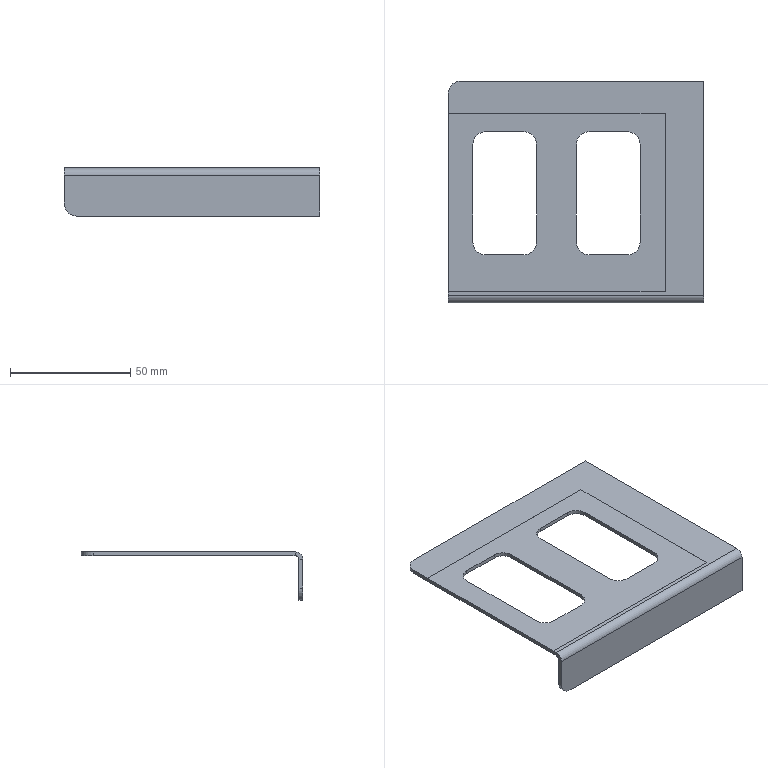Part | SolidWorks | features ICE 3, Fillet 1, FlatPattern 1, SMBaseFlange 1, SheetMetal 1 | 1 solid | 40 faces | box 106 x 92 x 20 mm | volume 14216 mm3 | plane 28 | cylinder 12 | commonest cylinder face diameters 10.4 x8 10 x2 3 x1 6.2 x1
STEP:
#1=CARTESIAN_POINT('',(15.4,19.9,-0.01));
#2=VERTEX_POINT('',#1);
#3=CARTESIAN_POINT('',(10.2,25.1,-0.01));
#4=VERTEX_POINT('',#3);
#5=CARTESIAN_POINT('',(15.4,25.1,-0.01));
#6=DIRECTION('',(0.,0.,-1.));
#7=DIRECTION('',(1.,0.,0.));
#8=AXIS2_PLACEMENT_3D('',#5,#6,#7);
#9=CIRCLE('',#8,5.2);
#10=EDGE_CURVE('',#2,#4,#9,.T.);
#11=ORIENTED_EDGE('',*,*,#10,.F.);
#12=CARTESIAN_POINT('',(15.4,19.9,-1.59));
#13=VERTEX_POINT('',#12);
#14=CARTESIAN_POINT('',(15.4,19.9,-20.001));
#15=DIRECTION('',(0.,0.,1.));
#16=VECTOR('',#15,1000.);
#17=LINE('',#14,#16);
#18=EDGE_CURVE('',#13,#2,#17,.T.);
#19=ORIENTED_EDGE('',*,*,#18,.F.);
#20=CARTESIAN_POINT('',(10.2,25.1,-1.59));
#21=VERTEX_POINT('',#20);
#22=CARTESIAN_POINT('',(15.4,25.1,-1.59));
#23=DIRECTION('',(0.,0.,-1.));
#24=DIRECTION('',(1.,0.,0.));
#25=AXIS2_PLACEMENT_3D('',#22,#23,#24);
#26=CIRCLE('',#25,5.2);
#27=EDGE_CURVE('',#13,#21,#26,.T.);
#28=ORIENTED_EDGE('',*,*,#27,.T.);
#29=CARTESIAN_POINT('',(10.2,25.1,-20.001));
#30=DIRECTION('',(0.,0.,1.));
#31=VECTOR('',#30,1000.);
#32=LINE('',#29,#31);
#33=EDGE_CURVE('',#21,#4,#32,.T.);
#34=ORIENTED_EDGE('',*,*,#33,.T.);
#35=EDGE_LOOP('',(#11,#19,#28,#34));
#36=FACE_OUTER_BOUND('',#35,.T.);
#37=CARTESIAN_POINT('',(15.4,25.1,-20.001));
#38=DIRECTION('',(0.,0.,1.));
#39=DIRECTION('',(1.,0.,0.));
#40=AXIS2_PLACEMENT_3D('',#37,#38,#39);
#41=CYLINDRICAL_SURFACE('',#40,5.2);
#42=ADVANCED_FACE('',(#36),#41,.F.);
#43=CARTESIAN_POINT('',(10.2,65.8,-0.01));
#44=VERTEX_POINT('',#43);
#45=CARTESIAN_POINT('',(10.2,65.8,-0.01));
#46=DIRECTION('',(0.,1.,0.));
#47=VECTOR('',#46,1000.);
#48=LINE('',#45,#47);
#49=EDGE_CURVE('',#4,#44,#48,.T.);
#50=ORIENTED_EDGE('',*,*,#49,.F.);
#51=ORIENTED_EDGE('',*,*,#33,.F.);
#52=CARTESIAN_POINT('',(10.2,65.8,-1.59));
#53=VERTEX_POINT('',#52);
#54=CARTESIAN_POINT('',(10.2,65.8,-1.59));
#55=DIRECTION('',(0.,1.,0.));
#56=VECTOR('',#55,1000.);
#57=LINE('',#54,#56);
#58=EDGE_CURVE('',#21,#53,#57,.T.);
#59=ORIENTED_EDGE('',*,*,#58,.T.);
#60=CARTESIAN_POINT('',(10.2,65.8,-20.001));
#61=DIRECTION('',(0.,0.,1.));
#62=VECTOR('',#61,1000.);
#63=LINE('',#60,#62);
#64=EDGE_CURVE('',#53,#44,#63,.T.);
#65=ORIENTED_EDGE('',*,*,#64,.T.);
#66=EDGE_LOOP('',(#50,#51,#59,#65));
#67=FACE_OUTER_BOUND('',#66,.T.);
#68=CARTESIAN_POINT('',(10.2,65.8,-20.001));
#69=DIRECTION('',(-1.,0.,0.));
#70=DIRECTION('',(0.,-1.,0.));
#71=AXIS2_PLACEMENT_3D('',#68,#69,#70);
#72=PLANE('',#71);
#73=ADVANCED_FACE('',(#67),#72,.F.);
#74=CARTESIAN_POINT('',(15.4,71.,-0.01));
#75=VERTEX_POINT('',#74);
#76=CARTESIAN_POINT('',(15.4,65.8,-0.01));
#77=DIRECTION('',(0.,0.,-1.));
#78=DIRECTION('',(1.,0.,0.));
#79=AXIS2_PLACEMENT_3D('',#76,#77,#78);
#80=CIRCLE('',#79,5.2);
#81=EDGE_CURVE('',#44,#75,#80,.T.);
#82=ORIENTED_EDGE('',*,*,#81,.F.);
#83=ORIENTED_EDGE('',*,*,#64,.F.);
#84=CARTESIAN_POINT('',(15.4,71.,-1.59));
#85=VERTEX_POINT('',#84);
#86=CARTESIAN_POINT('',(15.4,65.8,-1.59));
#87=DIRECTION('',(0.,0.,-1.));
#88=DIRECTION('',(1.,0.,0.));
#89=AXIS2_PLACEMENT_3D('',#86,#87,#88);
#90=CIRCLE('',#89,5.2);
#91=EDGE_CURVE('',#53,#85,#90,.T.);
#92=ORIENTED_EDGE('',*,*,#91,.T.);
#93=CARTESIAN_POINT('',(15.4,71.,-20.001));
#94=DIRECTION('',(0.,0.,1.));
#95=VECTOR('',#94,1000.);
#96=LINE('',#93,#95);
#97=EDGE_CURVE('',#85,#75,#96,.T.);
#98=ORIENTED_EDGE('',*,*,#97,.T.);
#99=EDGE_LOOP('',(#82,#83,#92,#98));
#100=FACE_OUTER_BOUND('',#99,.T.);
#101=CARTESIAN_POINT('',(15.4,65.8,-20.001));
#102=DIRECTION('',(0.,0.,1.));
#103=DIRECTION('',(1.,0.,0.));
#104=AXIS2_PLACEMENT_3D('',#101,#102,#103);
#105=CYLINDRICAL_SURFACE('',#104,5.2);
#106=ADVANCED_FACE('',(#100),#105,.F.);
#107=CARTESIAN_POINT('',(31.4,71.,-0.01));
#108=VERTEX_POINT('',#107);
#109=CARTESIAN_POINT('',(15.4,71.,-0.01));
#110=DIRECTION('',(1.,0.,0.));
#111=VECTOR('',#110,1000.);
#112=LINE('',#109,#111);
#113=EDGE_CURVE('',#75,#108,#112,.T.);
#114=ORIENTED_EDGE('',*,*,#113,.F.);
#115=ORIENTED_EDGE('',*,*,#97,.F.);
#116=CARTESIAN_POINT('',(31.4,71.,-1.59));
#117=VERTEX_POINT('',#116);
#118=CARTESIAN_POINT('',(15.4,71.,-1.59));
#119=DIRECTION('',(1.,0.,0.));
#120=VECTOR('',#119,1000.);
#121=LINE('',#118,#120);
#122=EDGE_CURVE('',#85,#117,#121,.T.);
#123=ORIENTED_EDGE('',*,*,#122,.T.);
#124=CARTESIAN_POINT('',(31.4,71.,-20.001));
#125=DIRECTION('',(0.,0.,1.));
#126=VECTOR('',#125,1000.);
#127=LINE('',#124,#126);
#128=EDGE_CURVE('',#117,#108,#127,.T.);
#129=ORIENTED_EDGE('',*,*,#128,.T.);
#130=EDGE_LOOP('',(#114,#115,#123,#129));
#131=FACE_OUTER_BOUND('',#130,.T.);
#132=CARTESIAN_POINT('',(15.4,71.,-20.001));
#133=DIRECTION('',(0.,1.,0.));
#134=DIRECTION('',(-1.,0.,0.));
#135=AXIS2_PLACEMENT_3D('',#132,#133,#134);
#136=PLANE('',#135);
#137=ADVANCED_FACE('',(#131),#136,.F.);
#138=CARTESIAN_POINT('',(36.6,65.8,-0.01));
#139=VERTEX_POINT('',#138);
#140=CARTESIAN_POINT('',(31.4,65.8,-0.01));
#141=DIRECTION('',(0.,0.,-1.));
#142=DIRECTION('',(1.,0.,0.));
#143=AXIS2_PLACEMENT_3D('',#140,#141,#142);
#144=CIRCLE('',#143,5.2);
#145=EDGE_CURVE('',#108,#139,#144,.T.);
#146=ORIENTED_EDGE('',*,*,#145,.F.);
#147=ORIENTED_EDGE('',*,*,#128,.F.);
#148=CARTESIAN_POINT('',(36.6,65.8,-1.59));
#149=VERTEX_POINT('',#148);
#150=CARTESIAN_POINT('',(31.4,65.8,-1.59));
#151=DIRECTION('',(0.,0.,-1.));
#152=DIRECTION('',(1.,0.,0.));
#153=AXIS2_PLACEMENT_3D('',#150,#151,#152);
#154=CIRCLE('',#153,5.2);
#155=EDGE_CURVE('',#117,#149,#154,.T.);
#156=ORIENTED_EDGE('',*,*,#155,.T.);
#157=CARTESIAN_POINT('',(36.6,65.8,-20.001));
#158=DIRECTION('',(0.,0.,1.));
#159=VECTOR('',#158,1000.);
#160=LINE('',#157,#159);
#161=EDGE_CURVE('',#149,#139,#160,.T.);
#162=ORIENTED_EDGE('',*,*,#161,.T.);
#163=EDGE_LOOP('',(#146,#147,#156,#162));
#164=FACE_OUTER_BOUND('',#163,.T.);
#165=CARTESIAN_POINT('',(31.4,65.8,-20.001));
#166=DIRECTION('',(0.,0.,1.));
#167=DIRECTION('',(1.,0.,0.));
#168=AXIS2_PLACEMENT_3D('',#165,#166,#167);
#169=CYLINDRICAL_SURFACE('',#168,5.2);
#170=ADVANCED_FACE('',(#164),#169,.F.);
#171=CARTESIAN_POINT('',(36.6,25.1,-0.01));
#172=VERTEX_POINT('',#171);
#173=CARTESIAN_POINT('',(36.6,65.8,-0.01));
#174=DIRECTION('',(0.,-1.,0.));
#175=VECTOR('',#174,1000.);
#176=LINE('',#173,#175);
#177=EDGE_CURVE('',#139,#172,#176,.T.);
#178=ORIENTED_EDGE('',*,*,#177,.F.);
#179=ORIENTED_EDGE('',*,*,#161,.F.);
#180=CARTESIAN_POINT('',(36.6,25.1,-1.59));
#181=VERTEX_POINT('',#180);
#182=CARTESIAN_POINT('',(36.6,65.8,-1.59));
#183=DIRECTION('',(0.,-1.,0.));
#184=VECTOR('',#183,1000.);
#185=LINE('',#182,#184);
#186=EDGE_CURVE('',#149,#181,#185,.T.);
#187=ORIENTED_EDGE('',*,*,#186,.T.);
#188=CARTESIAN_POINT('',(36.6,25.1,-20.001));
#189=DIRECTION('',(0.,0.,1.));
#190=VECTOR('',#189,1000.);
#191=LINE('',#188,#190);
#192=EDGE_CURVE('',#181,#172,#191,.T.);
#193=ORIENTED_EDGE('',*,*,#192,.T.);
#194=EDGE_LOOP('',(#178,#179,#187,#193));
#195=FACE_OUTER_BOUND('',#194,.T.);
#196=CARTESIAN_POINT('',(36.6,65.8,-20.001));
#197=DIRECTION('',(1.,0.,0.));
#198=DIRECTION('',(0.,1.,0.));
#199=AXIS2_PLACEMENT_3D('',#196,#197,#198);
#200=PLANE('',#199);
#201=ADVANCED_FACE('',(#195),#200,.F.);
#202=CARTESIAN_POINT('',(31.4,19.9,-0.01));
#203=VERTEX_POINT('',#202);
#204=CARTESIAN_POINT('',(31.4,25.1,-0.01));
#205=DIRECTION('',(0.,0.,-1.));
#206=DIRECTION('',(1.,0.,0.));
#207=AXIS2_PLACEMENT_3D('',#204,#205,#206);
#208=CIRCLE('',#207,5.2);
#209=EDGE_CURVE('',#172,#203,#208,.T.);
#210=ORIENTED_EDGE('',*,*,#209,.F.);
#211=ORIENTED_EDGE('',*,*,#192,.F.);
#212=CARTESIAN_POINT('',(31.4,19.9,-1.59));
#213=VERTEX_POINT('',#212);
#214=CARTESIAN_POINT('',(31.4,25.1,-1.59));
#215=DIRECTION('',(0.,0.,-1.));
#216=DIRECTION('',(1.,0.,0.));
#217=AXIS2_PLACEMENT_3D('',#214,#215,#216);
#218=CIRCLE('',#217,5.2);
#219=EDGE_CURVE('',#181,#213,#218,.T.);
#220=ORIENTED_EDGE('',*,*,#219,.T.);
#221=CARTESIAN_POINT('',(31.4,19.9,-20.001));
#222=DIRECTION('',(0.,0.,1.));
#223=VECTOR('',#222,1000.);
#224=LINE('',#221,#223);
#225=EDGE_CURVE('',#213,#203,#224,.T.);
#226=ORIENTED_EDGE('',*,*,#225,.T.);
#227=EDGE_LOOP('',(#210,#211,#220,#226));
#228=FACE_OUTER_BOUND('',#227,.T.);
#229=CARTESIAN_POINT('',(31.4,25.1,-20.001));
#230=DIRECTION('',(0.,0.,1.));
#231=DIRECTION('',(1.,0.,0.));
#232=AXIS2_PLACEMENT_3D('',#229,#230,#231);
#233=CYLINDRICAL_SURFACE('',#232,5.2);
#234=ADVANCED_FACE('',(#228),#233,.F.);
#235=CARTESIAN_POINT('',(15.4,19.9,-0.01));
#236=DIRECTION('',(-1.,0.,0.));
#237=VECTOR('',#236,1000.);
#238=LINE('',#235,#237);
#239=EDGE_CURVE('',#203,#2,#238,.T.);
#240=ORIENTED_EDGE('',*,*,#239,.F.);
#241=ORIENTED_EDGE('',*,*,#225,.F.);
#242=CARTESIAN_POINT('',(15.4,19.9,-1.59));
#243=DIRECTION('',(-1.,0.,0.));
#244=VECTOR('',#243,1000.);
#245=LINE('',#242,#244);
#246=EDGE_CURVE('',#213,#13,#245,.T.);
#247=ORIENTED_EDGE('',*,*,#246,.T.);
#248=ORIENTED_EDGE('',*,*,#18,.T.);
#249=EDGE_LOOP('',(#240,#241,#247,#248));
#250=FACE_OUTER_BOUND('',#249,.T.);
#251=CARTESIAN_POINT('',(15.4,19.9,-20.001));
#252=DIRECTION('',(0.,-1.,0.));
#253=DIRECTION('',(0.,0.,-1.));
#254=AXIS2_PLACEMENT_3D('',#251,#252,#253);
#255=PLANE('',#254);
#256=ADVANCED_FACE('',(#250),#255,.F.);
#257=CARTESIAN_POINT('',(79.6,25.1,-0.01));
#258=VERTEX_POINT('',#257);
#259=CARTESIAN_POINT('',(74.4,19.9,-0.01));
#260=VERTEX_POINT('',#259);
#261=CARTESIAN_POINT('',(74.4,25.1,-0.01));
#262=DIRECTION('',(0.,0.,-1.));
#263=DIRECTION('',(1.,0.,0.));
#264=AXIS2_PLACEMENT_3D('',#261,#262,#263);
#265=CIRCLE('',#264,5.2);
#266=EDGE_CURVE('',#258,#260,#265,.T.);
#267=ORIENTED_EDGE('',*,*,#266,.F.);
#268=CARTESIAN_POINT('',(79.6,25.1,-1.59));
#269=VERTEX_POINT('',#268);
#270=CARTESIAN_POINT('',(79.6,25.1,-20.001));
#271=DIRECTION('',(0.,0.,1.));
#272=VECTOR('',#271,1000.);
#273=LINE('',#270,#272);
#274=EDGE_CURVE('',#269,#258,#273,.T.);
#275=ORIENTED_EDGE('',*,*,#274,.F.);
#276=CARTESIAN_POINT('',(74.4,19.9,-1.59));
#277=VERTEX_POINT('',#276);
#278=CARTESIAN_POINT('',(74.4,25.1,-1.59));
#279=DIRECTION('',(0.,0.,-1.));
#280=DIRECTION('',(1.,0.,0.));
#281=AXIS2_PLACEMENT_3D('',#278,#279,#280);
#282=CIRCLE('',#281,5.2);
#283=EDGE_CURVE('',#269,#277,#282,.T.);
#284=ORIENTED_EDGE('',*,*,#283,.T.);
#285=CARTESIAN_POINT('',(74.4,19.9,-20.001));
#286=DIRECTION('',(0.,0.,1.));
#287=VECTOR('',#286,1000.);
#288=LINE('',#285,#287);
#289=EDGE_CURVE('',#277,#260,#288,.T.);
#290=ORIENTED_EDGE('',*,*,#289,.T.);
#291=EDGE_LOOP('',(#267,#275,#284,#290));
#292=FACE_OUTER_BOUND('',#291,.T.);
#293=CARTESIAN_POINT('',(74.4,25.1,-20.001));
#294=DIRECTION('',(0.,0.,1.));
#295=DIRECTION('',(1.,0.,0.));
#296=AXIS2_PLACEMENT_3D('',#293,#294,#295);
#297=CYLINDRICAL_SURFACE('',#296,5.2);
#298=ADVANCED_FACE('',(#292),#297,.F.);
#299=CARTESIAN_POINT('',(58.4,19.9,-0.01));
#300=VERTEX_POINT('',#299);
#301=CARTESIAN_POINT('',(58.4,19.9,-0.01));
#302=DIRECTION('',(-1.,0.,0.));
#303=VECTOR('',#302,1000.);
#304=LINE('',#301,#303);
#305=EDGE_CURVE('',#260,#300,#304,.T.);
#306=ORIENTED_EDGE('',*,*,#305,.F.);
#307=ORIENTED_EDGE('',*,*,#289,.F.);
#308=CARTESIAN_POINT('',(58.4,19.9,-1.59));
#309=VERTEX_POINT('',#308);
#310=CARTESIAN_POINT('',(58.4,19.9,-1.59));
#311=DIRECTION('',(-1.,0.,0.));
#312=VECTOR('',#311,1000.);
#313=LINE('',#310,#312);
#314=EDGE_CURVE('',#277,#309,#313,.T.);
#315=ORIENTED_EDGE('',*,*,#314,.T.);
#316=CARTESIAN_POINT('',(58.4,19.9,-20.001));
#317=DIRECTION('',(0.,0.,1.));
#318=VECTOR('',#317,1000.);
#319=LINE('',#316,#318);
#320=EDGE_CURVE('',#309,#300,#319,.T.);
#321=ORIENTED_EDGE('',*,*,#320,.T.);
#322=EDGE_LOOP('',(#306,#307,#315,#321));
#323=FACE_OUTER_BOUND('',#322,.T.);
#324=CARTESIAN_POINT('',(58.4,19.9,-20.001));
#325=DIRECTION('',(0.,-1.,0.));
#326=DIRECTION('',(0.,0.,-1.));
#327=AXIS2_PLACEMENT_3D('',#324,#325,#326);
#328=PLANE('',#327);
#329=ADVANCED_FACE('',(#323),#328,.F.);
#330=CARTESIAN_POINT('',(53.2,25.1,-0.01));
#331=VERTEX_POINT('',#330);
#332=CARTESIAN_POINT('',(58.4,25.1,-0.01));
#333=DIRECTION('',(0.,0.,-1.));
#334=DIRECTION('',(1.,0.,0.));
#335=AXIS2_PLACEMENT_3D('',#332,#333,#334);
#336=CIRCLE('',#335,5.2);
#337=EDGE_CURVE('',#300,#331,#336,.T.);
#338=ORIENTED_EDGE('',*,*,#337,.F.);
#339=ORIENTED_EDGE('',*,*,#320,.F.);
#340=CARTESIAN_POINT('',(53.2,25.1,-1.59));
#341=VERTEX_POINT('',#340);
#342=CARTESIAN_POINT('',(58.4,25.1,-1.59));
#343=DIRECTION('',(0.,0.,-1.));
#344=DIRECTION('',(1.,0.,0.));
#345=AXIS2_PLACEMENT_3D('',#342,#343,#344);
#346=CIRCLE('',#345,5.2);
#347=EDGE_CURVE('',#309,#341,#346,.T.);
#348=ORIENTED_EDGE('',*,*,#347,.T.);
#349=CARTESIAN_POINT('',(53.2,25.1,-20.001));
#350=DIRECTION('',(0.,0.,1.));
#351=VECTOR('',#350,1000.);
#352=LINE('',#349,#351);
#353=EDGE_CURVE('',#341,#331,#352,.T.);
#354=ORIENTED_EDGE('',*,*,#353,.T.);
#355=EDGE_LOOP('',(#338,#339,#348,#354));
#356=FACE_OUTER_BOUND('',#355,.T.);
#357=CARTESIAN_POINT('',(58.4,25.1,-20.001));
#358=DIRECTION('',(0.,0.,1.));
#359=DIRECTION('',(1.,0.,0.));
#360=AXIS2_PLACEMENT_3D('',#357,#358,#359);
#361=CYLINDRICAL_SURFACE('',#360,5.2);
#362=ADVANCED_FACE('',(#356),#361,.F.);
#363=CARTESIAN_POINT('',(53.2,65.8,-0.01));
#364=VERTEX_POINT('',#363);
#365=CARTESIAN_POINT('',(53.2,65.8,-0.01));
#366=DIRECTION('',(0.,1.,0.));
#367=VECTOR('',#366,1000.);
#368=LINE('',#365,#367);
#369=EDGE_CURVE('',#331,#364,#368,.T.);
#370=ORIENTED_EDGE('',*,*,#369,.F.);
#371=ORIENTED_EDGE('',*,*,#353,.F.);
#372=CARTESIAN_POINT('',(53.2,65.8,-1.59));
#373=VERTEX_POINT('',#372);
#374=CARTESIAN_POINT('',(53.2,65.8,-1.59));
#375=DIRECTION('',(0.,1.,0.));
#376=VECTOR('',#375,1000.);
#377=LINE('',#374,#376);
#378=EDGE_CURVE('',#341,#373,#377,.T.);
#379=ORIENTED_EDGE('',*,*,#378,.T.);
#380=CARTESIAN_POINT('',(53.2,65.8,-20.001));
#381=DIRECTION('',(0.,0.,1.));
#382=VECTOR('',#381,1000.);
#383=LINE('',#380,#382);
#384=EDGE_CURVE('',#373,#364,#383,.T.);
#385=ORIENTED_EDGE('',*,*,#384,.T.);
#386=EDGE_LOOP('',(#370,#371,#379,#385));
#387=FACE_OUTER_BOUND('',#386,.T.);
#388=CARTESIAN_POINT('',(53.2,65.8,-20.001));
#389=DIRECTION('',(-1.,0.,0.));
#390=DIRECTION('',(0.,-1.,0.));
#391=AXIS2_PLACEMENT_3D('',#388,#389,#390);
#392=PLANE('',#391);
#393=ADVANCED_FACE('',(#387),#392,.F.);
#394=CARTESIAN_POINT('',(58.4,71.,-0.01));
#395=VERTEX_POINT('',#394);
#396=CARTESIAN_POINT('',(58.4,65.8,-0.01));
#397=DIRECTION('',(0.,0.,-1.));
#398=DIRECTION('',(1.,0.,0.));
#399=AXIS2_PLACEMENT_3D('',#396,#397,#398);
#400=CIRCLE('',#399,5.2);
#401=EDGE_CURVE('',#364,#395,#400,.T.);
#402=ORIENTED_EDGE('',*,*,#401,.F.);
#403=ORIENTED_EDGE('',*,*,#384,.F.);
#404=CARTESIAN_POINT('',(58.4,71.,-1.59));
#405=VERTEX_POINT('',#404);
#406=CARTESIAN_POINT('',(58.4,65.8,-1.59));
#407=DIRECTION('',(0.,0.,-1.));
#408=DIRECTION('',(1.,0.,0.));
#409=AXIS2_PLACEMENT_3D('',#406,#407,#408);
#410=CIRCLE('',#409,5.2);
#411=EDGE_CURVE('',#373,#405,#410,.T.);
#412=ORIENTED_EDGE('',*,*,#411,.T.);
#413=CARTESIAN_POINT('',(58.4,71.,-20.001));
#414=DIRECTION('',(0.,0.,1.));
#415=VECTOR('',#414,1000.);
#416=LINE('',#413,#415);
#417=EDGE_CURVE('',#405,#395,#416,.T.);
#418=ORIENTED_EDGE('',*,*,#417,.T.);
#419=EDGE_LOOP('',(#402,#403,#412,#418));
#420=FACE_OUTER_BOUND('',#419,.T.);
#421=CARTESIAN_POINT('',(58.4,65.8,-20.001));
#422=DIRECTION('',(0.,0.,1.));
#423=DIRECTION('',(1.,0.,0.));
#424=AXIS2_PLACEMENT_3D('',#421,#422,#423);
#425=CYLINDRICAL_SURFACE('',#424,5.2);
#426=ADVANCED_FACE('',(#420),#425,.F.);
#427=CARTESIAN_POINT('',(74.4,71.,-0.01));
#428=VERTEX_POINT('',#427);
#429=CARTESIAN_POINT('',(58.4,71.,-0.01));
#430=DIRECTION('',(1.,0.,0.));
#431=VECTOR('',#430,1000.);
#432=LINE('',#429,#431);
#433=EDGE_CURVE('',#395,#428,#432,.T.);
#434=ORIENTED_EDGE('',*,*,#433,.F.);
#435=ORIENTED_EDGE('',*,*,#417,.F.);
#436=CARTESIAN_POINT('',(74.4,71.,-1.59));
#437=VERTEX_POINT('',#436);
#438=CARTESIAN_POINT('',(58.4,71.,-1.59));
#439=DIRECTION('',(1.,0.,0.));
#440=VECTOR('',#439,1000.);
#441=LINE('',#438,#440);
#442=EDGE_CURVE('',#405,#437,#441,.T.);
#443=ORIENTED_EDGE('',*,*,#442,.T.);
#444=CARTESIAN_POINT('',(74.4,71.,-20.001));
#445=DIRECTION('',(0.,0.,1.));
#446=VECTOR('',#445,1000.);
#447=LINE('',#444,#446);
#448=EDGE_CURVE('',#437,#428,#447,.T.);
#449=ORIENTED_EDGE('',*,*,#448,.T.);
#450=EDGE_LOOP('',(#434,#435,#443,#449));
#451=FACE_OUTER_BOUND('',#450,.T.);
#452=CARTESIAN_POINT('',(58.4,71.,-20.001));
#453=DIRECTION('',(0.,1.,0.));
#454=DIRECTION('',(0.,0.,1.));
#455=AXIS2_PLACEMENT_3D('',#452,#453,#454);
#456=PLANE('',#455);
#457=ADVANCED_FACE('',(#451),#456,.F.);
#458=CARTESIAN_POINT('',(79.6,65.8,-0.01));
#459=VERTEX_POINT('',#458);
#460=CARTESIAN_POINT('',(74.4,65.8,-0.01));
#461=DIRECTION('',(0.,0.,-1.));
#462=DIRECTION('',(1.,0.,0.));
#463=AXIS2_PLACEMENT_3D('',#460,#461,#462);
#464=CIRCLE('',#463,5.2);
#465=EDGE_CURVE('',#428,#459,#464,.T.);
#466=ORIENTED_EDGE('',*,*,#465,.F.);
#467=ORIENTED_EDGE('',*,*,#448,.F.);
#468=CARTESIAN_POINT('',(79.6,65.8,-1.59));
#469=VERTEX_POINT('',#468);
#470=CARTESIAN_POINT('',(74.4,65.8,-1.59));
#471=DIRECTION('',(0.,0.,-1.));
#472=DIRECTION('',(1.,0.,0.));
#473=AXIS2_PLACEMENT_3D('',#470,#471,#472);
#474=CIRCLE('',#473,5.2);
#475=EDGE_CURVE('',#437,#469,#474,.T.);
#476=ORIENTED_EDGE('',*,*,#475,.T.);
#477=CARTESIAN_POINT('',(79.6,65.8,-20.001));
#478=DIRECTION('',(0.,0.,1.));
#479=VECTOR('',#478,1000.);
#480=LINE('',#477,#479);
#481=EDGE_CURVE('',#469,#459,#480,.T.);
#482=ORIENTED_EDGE('',*,*,#481,.T.);
#483=EDGE_LOOP('',(#466,#467,#476,#482));
#484=FACE_OUTER_BOUND('',#483,.T.);
#485=CARTESIAN_POINT('',(74.4,65.8,-20.001));
#486=DIRECTION('',(0.,0.,1.));
#487=DIRECTION('',(1.,0.,0.));
#488=AXIS2_PLACEMENT_3D('',#485,#486,#487);
#489=CYLINDRICAL_SURFACE('',#488,5.2);
#490=ADVANCED_FACE('',(#484),#489,.F.);
#491=CARTESIAN_POINT('',(79.6,65.8,-0.01));
#492=DIRECTION('',(0.,-1.,0.));
#493=VECTOR('',#492,1000.);
#494=LINE('',#491,#493);
#495=EDGE_CURVE('',#459,#258,#494,.T.);
#496=ORIENTED_EDGE('',*,*,#495,.F.);
#497=ORIENTED_EDGE('',*,*,#481,.F.);
#498=CARTESIAN_POINT('',(79.6,65.8,-1.59));
#499=DIRECTION('',(0.,-1.,0.));
#500=VECTOR('',#499,1000.);
#501=LINE('',#498,#500);
#502=EDGE_CURVE('',#469,#269,#501,.T.);
#503=ORIENTED_EDGE('',*,*,#502,.T.);
#504=ORIENTED_EDGE('',*,*,#274,.T.);
#505=EDGE_LOOP('',(#496,#497,#503,#504));
#506=FACE_OUTER_BOUND('',#505,.T.);
#507=CARTESIAN_POINT('',(79.6,65.8,-20.001));
#508=DIRECTION('',(1.,0.,0.));
#509=DIRECTION('',(0.,0.,-1.));
#510=AXIS2_PLACEMENT_3D('',#507,#508,#509);
#511=PLANE('',#510);
#512=ADVANCED_FACE('',(#506),#511,.F.);
#513=CARTESIAN_POINT('',(106.,3.1,0.));
#514=VERTEX_POINT('',#513);
#515=CARTESIAN_POINT('',(106.,3.1,-1.6));
#516=VERTEX_POINT('',#515);
#517=CARTESIAN_POINT('',(106.,3.1,0.));
#518=DIRECTION('',(0.,0.,-1.));
#519=VECTOR('',#518,1000.);
#520=LINE('',#517,#519);
#521=EDGE_CURVE('',#514,#516,#520,.T.);
#522=ORIENTED_EDGE('',*,*,#521,.F.);
#523=CARTESIAN_POINT('',(106.,0.,-3.1));
#524=VERTEX_POINT('',#523);
#525=CARTESIAN_POINT('',(106.,3.1,-3.1));
#526=DIRECTION('',(-1.,0.,0.));
#527=DIRECTION('',(0.,0.,-1.));
#528=AXIS2_PLACEMENT_3D('',#525,#526,#527);
#529=CIRCLE('',#528,3.1);
#530=EDGE_CURVE('',#524,#514,#529,.T.);
#531=ORIENTED_EDGE('',*,*,#530,.F.);
#532=CARTESIAN_POINT('',(106.,1.6,-3.1));
#533=VERTEX_POINT('',#532);
#534=CARTESIAN_POINT('',(106.,1.6,-3.1));
#535=DIRECTION('',(0.,-1.,0.));
#536=VECTOR('',#535,1000.);
#537=LINE('',#534,#536);
#538=EDGE_CURVE('',#533,#524,#537,.T.);
#539=ORIENTED_EDGE('',*,*,#538,.F.);
#540=CARTESIAN_POINT('',(106.,3.1,-3.1));
#541=DIRECTION('',(-1.,0.,0.));
#542=DIRECTION('',(0.,0.,-1.));
#543=AXIS2_PLACEMENT_3D('',#540,#541,#542);
#544=CIRCLE('',#543,1.5);
#545=EDGE_CURVE('',#533,#516,#544,.T.);
#546=ORIENTED_EDGE('',*,*,#545,.T.);
#547=EDGE_LOOP('',(#522,#531,#539,#546));
#548=FACE_OUTER_BOUND('',#547,.T.);
#549=CARTESIAN_POINT('',(106.,3.1,0.));
#550=DIRECTION('',(1.,0.,0.));
#551=DIRECTION('',(0.,0.,-1.));
#552=AXIS2_PLACEMENT_3D('',#549,#550,#551);
#553=PLANE('',#552);
#554=ADVANCED_FACE('',(#548),#553,.T.);
#555=CARTESIAN_POINT('',(106.,92.,0.));
#556=VERTEX_POINT('',#555);
#557=CARTESIAN_POINT('',(106.,0.,0.));
#558=DIRECTION('',(0.,1.,0.));
#559=VECTOR('',#558,1000.);
#560=LINE('',#557,#559);
#561=EDGE_CURVE('',#514,#556,#560,.T.);
#562=ORIENTED_EDGE('',*,*,#561,.F.);
#563=ORIENTED_EDGE('',*,*,#521,.T.);
#564=CARTESIAN_POINT('',(106.,92.,-1.6));
#565=VERTEX_POINT('',#564);
#566=CARTESIAN_POINT('',(106.,0.,-1.6));
#567=DIRECTION('',(0.,1.,0.));
#568=VECTOR('',#567,1000.);
#569=LINE('',#566,#568);
#570=EDGE_CURVE('',#516,#565,#569,.T.);
#571=ORIENTED_EDGE('',*,*,#570,.T.);
#572=CARTESIAN_POINT('',(106.,92.,0.));
#573=DIRECTION('',(0.,0.,-1.));
#574=VECTOR('',#573,1000.);
#575=LINE('',#572,#574);
#576=EDGE_CURVE('',#556,#565,#575,.T.);
#577=ORIENTED_EDGE('',*,*,#576,.F.);
#578=EDGE_LOOP('',(#562,#563,#571,#577));
#579=FACE_OUTER_BOUND('',#578,.T.);
#580=CARTESIAN_POINT('',(106.,1.6,-3.1));
#581=DIRECTION('',(1.,0.,0.));
#582=DIRECTION('',(0.,0.,-1.));
#583=AXIS2_PLACEMENT_3D('',#580,#581,#582);
#584=PLANE('',#583);
#585=ADVANCED_FACE('',(#579),#584,.T.);
#586=CARTESIAN_POINT('',(0.,0.,-3.1));
#587=VERTEX_POINT('',#586);
#588=CARTESIAN_POINT('',(0.,1.6,-3.1));
#589=VERTEX_POINT('',#588);
#590=CARTESIAN_POINT('',(0.,0.,-3.1));
#591=DIRECTION('',(0.,1.,0.));
#592=VECTOR('',#591,1000.);
#593=LINE('',#590,#592);
#594=EDGE_CURVE('',#587,#589,#593,.T.);
#595=ORIENTED_EDGE('',*,*,#594,.F.);
#596=CARTESIAN_POINT('',(0.,3.1,0.));
#597=VERTEX_POINT('',#596);
#598=CARTESIAN_POINT('',(0.,3.1,-3.1));
#599=DIRECTION('',(-1.,0.,0.));
#600=DIRECTION('',(0.,0.,-1.));
#601=AXIS2_PLACEMENT_3D('',#598,#599,#600);
#602=CIRCLE('',#601,3.1);
#603=EDGE_CURVE('',#587,#597,#602,.T.);
#604=ORIENTED_EDGE('',*,*,#603,.T.);
#605=CARTESIAN_POINT('',(0.,3.1,-1.6));
#606=VERTEX_POINT('',#605);
#607=CARTESIAN_POINT('',(0.,3.1,-1.6));
#608=DIRECTION('',(0.,0.,1.));
#609=VECTOR('',#608,1000.);
#610=LINE('',#607,#609);
#611=EDGE_CURVE('',#606,#597,#610,.T.);
#612=ORIENTED_EDGE('',*,*,#611,.F.);
#613=CARTESIAN_POINT('',(0.,3.1,-3.1));
#614=DIRECTION('',(-1.,0.,0.));
#615=DIRECTION('',(0.,0.,-1.));
#616=AXIS2_PLACEMENT_3D('',#613,#614,#615);
#617=CIRCLE('',#616,1.5);
#618=EDGE_CURVE('',#589,#606,#617,.T.);
#619=ORIENTED_EDGE('',*,*,#618,.F.);
#620=EDGE_LOOP('',(#595,#604,#612,#619));
#621=FACE_OUTER_BOUND('',#620,.T.);
#622=CARTESIAN_POINT('',(0.,0.,-3.1));
#623=DIRECTION('',(-1.,0.,0.));
#624=DIRECTION('',(0.,0.,1.));
#625=AXIS2_PLACEMENT_3D('',#622,#623,#624);
#626=PLANE('',#625);
#627=ADVANCED_FACE('',(#621),#626,.T.);
#628=CARTESIAN_POINT('',(0.,1.6,-15.));
#629=VERTEX_POINT('',#628);
#630=CARTESIAN_POINT('',(0.,1.6,-20.));
#631=DIRECTION('',(0.,0.,1.));
#632=VECTOR('',#631,1000.);
#633=LINE('',#630,#632);
#634=EDGE_CURVE('',#629,#589,#633,.T.);
#635=ORIENTED_EDGE('',*,*,#634,.F.);
#636=CARTESIAN_POINT('',(0.,0.,-15.));
#637=VERTEX_POINT('',#636);
#638=CARTESIAN_POINT('',(0.,3.1,-15.));
#639=DIRECTION('',(0.,-1.,0.));
#640=VECTOR('',#639,1000.);
#641=LINE('',#638,#640);
#642=EDGE_CURVE('',#629,#637,#641,.T.);
#643=ORIENTED_EDGE('',*,*,#642,.T.);
#644=CARTESIAN_POINT('',(0.,0.,-20.));
#645=DIRECTION('',(0.,0.,1.));
#646=VECTOR('',#645,1000.);
#647=LINE('',#644,#646);
#648=EDGE_CURVE('',#637,#587,#647,.T.);
#649=ORIENTED_EDGE('',*,*,#648,.T.);
#650=ORIENTED_EDGE('',*,*,#594,.T.);
#651=EDGE_LOOP('',(#635,#643,#649,#650));
#652=FACE_OUTER_BOUND('',#651,.T.);
#653=CARTESIAN_POINT('',(0.,3.1,-1.6));
#654=DIRECTION('',(-1.,0.,0.));
#655=DIRECTION('',(0.,0.,1.));
#656=AXIS2_PLACEMENT_3D('',#653,#654,#655);
#657=PLANE('',#656);
#658=ADVANCED_FACE('',(#652),#657,.T.);
#659=CARTESIAN_POINT('',(0.,4.6,-1.6));
#660=VERTEX_POINT('',#659);
#661=CARTESIAN_POINT('',(0.,0.,-1.6));
#662=DIRECTION('',(0.,1.,0.));
#663=VECTOR('',#662,1000.);
#664=LINE('',#661,#663);
#665=EDGE_CURVE('',#606,#660,#664,.T.);
#666=ORIENTED_EDGE('',*,*,#665,.T.);
#667=CARTESIAN_POINT('',(90.,4.6,-1.6));
#668=VERTEX_POINT('',#667);
#669=CARTESIAN_POINT('',(0.,4.6,-1.6));
#670=DIRECTION('',(-1.,0.,0.));
#671=VECTOR('',#670,1000.);
#672=LINE('',#669,#671);
#673=EDGE_CURVE('',#668,#660,#672,.T.);
#674=ORIENTED_EDGE('',*,*,#673,.F.);
#675=CARTESIAN_POINT('',(90.,78.6,-1.6));
#676=VERTEX_POINT('',#675);
#677=CARTESIAN_POINT('',(90.,78.6,-1.6));
#678=DIRECTION('',(0.,-1.,0.));
#679=VECTOR('',#678,1000.);
#680=LINE('',#677,#679);
#681=EDGE_CURVE('',#676,#668,#680,.T.);
#682=ORIENTED_EDGE('',*,*,#681,.F.);
#683=CARTESIAN_POINT('',(0.,78.6,-1.6));
#684=VERTEX_POINT('',#683);
#685=CARTESIAN_POINT('',(0.,78.6,-1.6));
#686=DIRECTION('',(1.,0.,0.));
#687=VECTOR('',#686,1000.);
#688=LINE('',#685,#687);
#689=EDGE_CURVE('',#684,#676,#688,.T.);
#690=ORIENTED_EDGE('',*,*,#689,.F.);
#691=CARTESIAN_POINT('',(0.,87.,-1.6));
#692=VERTEX_POINT('',#691);
#693=CARTESIAN_POINT('',(0.,0.,-1.6));
#694=DIRECTION('',(0.,1.,0.));
#695=VECTOR('',#694,1000.);
#696=LINE('',#693,#695);
#697=EDGE_CURVE('',#684,#692,#696,.T.);
#698=ORIENTED_EDGE('',*,*,#697,.T.);
#699=CARTESIAN_POINT('',(5.,92.,-1.6));
#700=VERTEX_POINT('',#699);
#701=CARTESIAN_POINT('',(5.,87.,-1.6));
#702=DIRECTION('',(0.,0.,-1.));
#703=DIRECTION('',(1.,0.,0.));
#704=AXIS2_PLACEMENT_3D('',#701,#702,#703);
#705=CIRCLE('',#704,5.);
#706=EDGE_CURVE('',#692,#700,#705,.T.);
#707=ORIENTED_EDGE('',*,*,#706,.T.);
#708=CARTESIAN_POINT('',(106.,92.,-1.6));
#709=DIRECTION('',(-1.,0.,0.));
#710=VECTOR('',#709,1000.);
#711=LINE('',#708,#710);
#712=EDGE_CURVE('',#565,#700,#711,.T.);
#713=ORIENTED_EDGE('',*,*,#712,.F.);
#714=ORIENTED_EDGE('',*,*,#570,.F.);
#715=CARTESIAN_POINT('',(106.,3.1,-1.6));
#716=DIRECTION('',(-1.,0.,0.));
#717=VECTOR('',#716,1000.);
#718=LINE('',#715,#717);
#719=EDGE_CURVE('',#516,#606,#718,.T.);
#720=ORIENTED_EDGE('',*,*,#719,.T.);
#721=EDGE_LOOP('',(#666,#674,#682,#690,#698,#707,#713,#714,#720));
#722=FACE_OUTER_BOUND('',#721,.T.);
#723=CARTESIAN_POINT('',(106.,0.,-1.6));
#724=DIRECTION('',(0.,0.,1.));
#725=DIRECTION('',(1.,0.,0.));
#726=AXIS2_PLACEMENT_3D('',#723,#724,#725);
#727=PLANE('',#726);
#728=ADVANCED_FACE('',(#722),#727,.F.);
#729=ORIENTED_EDGE('',*,*,#712,.T.);
#730=CARTESIAN_POINT('',(5.,92.,0.));
#731=VERTEX_POINT('',#730);
#732=CARTESIAN_POINT('',(5.,92.,0.));
#733=DIRECTION('',(0.,0.,1.));
#734=VECTOR('',#733,1000.);
#735=LINE('',#732,#734);
#736=EDGE_CURVE('',#700,#731,#735,.T.);
#737=ORIENTED_EDGE('',*,*,#736,.T.);
#738=CARTESIAN_POINT('',(106.,92.,0.));
#739=DIRECTION('',(-1.,0.,0.));
#740=VECTOR('',#739,1000.);
#741=LINE('',#738,#740);
#742=EDGE_CURVE('',#556,#731,#741,.T.);
#743=ORIENTED_EDGE('',*,*,#742,.F.);
#744=ORIENTED_EDGE('',*,*,#576,.T.);
#745=EDGE_LOOP('',(#729,#737,#743,#744));
#746=FACE_OUTER_BOUND('',#745,.T.);
#747=CARTESIAN_POINT('',(106.,92.,0.));
#748=DIRECTION('',(0.,1.,0.));
#749=DIRECTION('',(0.,0.,1.));
#750=AXIS2_PLACEMENT_3D('',#747,#748,#749);
#751=PLANE('',#750);
#752=ADVANCED_FACE('',(#746),#751,.T.);
#753=CARTESIAN_POINT('',(90.,78.6,0.));
#754=VERTEX_POINT('',#753);
#755=CARTESIAN_POINT('',(0.,78.6,0.));
#756=VERTEX_POINT('',#755);
#757=CARTESIAN_POINT('',(0.,78.6,0.));
#758=DIRECTION('',(-1.,0.,0.));
#759=VECTOR('',#758,1000.);
#760=LINE('',#757,#759);
#761=EDGE_CURVE('',#754,#756,#760,.T.);
#762=ORIENTED_EDGE('',*,*,#761,.F.);
#763=CARTESIAN_POINT('',(90.,4.6,0.));
#764=VERTEX_POINT('',#763);
#765=CARTESIAN_POINT('',(90.,78.6,0.));
#766=DIRECTION('',(0.,1.,0.));
#767=VECTOR('',#766,1000.);
#768=LINE('',#765,#767);
#769=EDGE_CURVE('',#764,#754,#768,.T.);
#770=ORIENTED_EDGE('',*,*,#769,.F.);
#771=CARTESIAN_POINT('',(0.,4.6,0.));
#772=VERTEX_POINT('',#771);
#773=CARTESIAN_POINT('',(0.,4.6,0.));
#774=DIRECTION('',(1.,0.,0.));
#775=VECTOR('',#774,1000.);
#776=LINE('',#773,#775);
#777=EDGE_CURVE('',#772,#764,#776,.T.);
#778=ORIENTED_EDGE('',*,*,#777,.F.);
#779=CARTESIAN_POINT('',(0.,0.,0.));
#780=DIRECTION('',(0.,1.,0.));
#781=VECTOR('',#780,1000.);
#782=LINE('',#779,#781);
#783=EDGE_CURVE('',#597,#772,#782,.T.);
#784=ORIENTED_EDGE('',*,*,#783,.F.);
#785=CARTESIAN_POINT('',(106.,3.1,0.));
#786=DIRECTION('',(-1.,0.,0.));
#787=VECTOR('',#786,1000.);
#788=LINE('',#785,#787);
#789=EDGE_CURVE('',#514,#597,#788,.T.);
#790=ORIENTED_EDGE('',*,*,#789,.F.);
#791=ORIENTED_EDGE('',*,*,#561,.T.);
#792=ORIENTED_EDGE('',*,*,#742,.T.);
#793=CARTESIAN_POINT('',(0.,87.,0.));
#794=VERTEX_POINT('',#793);
#795=CARTESIAN_POINT('',(5.,87.,0.));
#796=DIRECTION('',(0.,0.,1.));
#797=DIRECTION('',(1.,0.,0.));
#798=AXIS2_PLACEMENT_3D('',#795,#796,#797);
#799=CIRCLE('',#798,5.);
#800=EDGE_CURVE('',#731,#794,#799,.T.);
#801=ORIENTED_EDGE('',*,*,#800,.T.);
#802=CARTESIAN_POINT('',(0.,0.,0.));
#803=DIRECTION('',(0.,1.,0.));
#804=VECTOR('',#803,1000.);
#805=LINE('',#802,#804);
#806=EDGE_CURVE('',#756,#794,#805,.T.);
#807=ORIENTED_EDGE('',*,*,#806,.F.);
#808=EDGE_LOOP('',(#762,#770,#778,#784,#790,#791,#792,#801,#807));
#809=FACE_OUTER_BOUND('',#808,.T.);
#810=CARTESIAN_POINT('',(106.,0.,0.));
#811=DIRECTION('',(0.,0.,1.));
#812=DIRECTION('',(1.,0.,0.));
#813=AXIS2_PLACEMENT_3D('',#810,#811,#812);
#814=PLANE('',#813);
#815=ADVANCED_FACE('',(#809),#814,.T.);
#816=ORIENTED_EDGE('',*,*,#603,.F.);
#817=CARTESIAN_POINT('',(106.,0.,-3.1));
#818=DIRECTION('',(-1.,0.,0.));
#819=VECTOR('',#818,1000.);
#820=LINE('',#817,#819);
#821=EDGE_CURVE('',#524,#587,#820,.T.);
#822=ORIENTED_EDGE('',*,*,#821,.F.);
#823=ORIENTED_EDGE('',*,*,#530,.T.);
#824=ORIENTED_EDGE('',*,*,#789,.T.);
#825=EDGE_LOOP('',(#816,#822,#823,#824));
#826=FACE_OUTER_BOUND('',#825,.T.);
#827=CARTESIAN_POINT('',(106.,3.1,-3.1));
#828=DIRECTION('',(-1.,0.,0.));
#829=DIRECTION('',(0.,0.,1.));
#830=AXIS2_PLACEMENT_3D('',#827,#828,#829);
#831=CYLINDRICAL_SURFACE('',#830,3.1);
#832=ADVANCED_FACE('',(#826),#831,.T.);
#833=ORIENTED_EDGE('',*,*,#648,.F.);
#834=CARTESIAN_POINT('',(5.,0.,-20.));
#835=VERTEX_POINT('',#834);
#836=CARTESIAN_POINT('',(5.,0.,-15.));
#837=DIRECTION('',(0.,-1.,0.));
#838=DIRECTION('',(0.,0.,-1.));
#839=AXIS2_PLACEMENT_3D('',#836,#837,#838);
#840=CIRCLE('',#839,5.);
#841=EDGE_CURVE('',#637,#835,#840,.T.);
#842=ORIENTED_EDGE('',*,*,#841,.T.);
#843=CARTESIAN_POINT('',(106.,0.,-20.));
#844=VERTEX_POINT('',#843);
#845=CARTESIAN_POINT('',(106.,0.,-20.));
#846=DIRECTION('',(-1.,0.,0.));
#847=VECTOR('',#846,1000.);
#848=LINE('',#845,#847);
#849=EDGE_CURVE('',#844,#835,#848,.T.);
#850=ORIENTED_EDGE('',*,*,#849,.F.);
#851=CARTESIAN_POINT('',(106.,0.,-20.));
#852=DIRECTION('',(0.,0.,1.));
#853=VECTOR('',#852,1000.);
#854=LINE('',#851,#853);
#855=EDGE_CURVE('',#844,#524,#854,.T.);
#856=ORIENTED_EDGE('',*,*,#855,.T.);
#857=ORIENTED_EDGE('',*,*,#821,.T.);
#858=EDGE_LOOP('',(#833,#842,#850,#856,#857));
#859=FACE_OUTER_BOUND('',#858,.T.);
#860=CARTESIAN_POINT('',(106.,0.,-20.));
#861=DIRECTION('',(0.,-1.,0.));
#862=DIRECTION('',(0.,0.,-1.));
#863=AXIS2_PLACEMENT_3D('',#860,#861,#862);
#864=PLANE('',#863);
#865=ADVANCED_FACE('',(#859),#864,.T.);
#866=ORIENTED_EDGE('',*,*,#849,.T.);
#867=CARTESIAN_POINT('',(5.,1.6,-20.));
#868=VERTEX_POINT('',#867);
#869=CARTESIAN_POINT('',(5.,1.6,-20.));
#870=DIRECTION('',(0.,1.,0.));
#871=VECTOR('',#870,1000.);
#872=LINE('',#869,#871);
#873=EDGE_CURVE('',#835,#868,#872,.T.);
#874=ORIENTED_EDGE('',*,*,#873,.T.);
#875=CARTESIAN_POINT('',(106.,1.6,-20.));
#876=VERTEX_POINT('',#875);
#877=CARTESIAN_POINT('',(106.,1.6,-20.));
#878=DIRECTION('',(-1.,0.,0.));
#879=VECTOR('',#878,1000.);
#880=LINE('',#877,#879);
#881=EDGE_CURVE('',#876,#868,#880,.T.);
#882=ORIENTED_EDGE('',*,*,#881,.F.);
#883=CARTESIAN_POINT('',(106.,1.6,-20.));
#884=DIRECTION('',(0.,-1.,0.));
#885=VECTOR('',#884,1000.);
#886=LINE('',#883,#885);
#887=EDGE_CURVE('',#876,#844,#886,.T.);
#888=ORIENTED_EDGE('',*,*,#887,.T.);
#889=EDGE_LOOP('',(#866,#874,#882,#888));
#890=FACE_OUTER_BOUND('',#889,.T.);
#891=CARTESIAN_POINT('',(106.,1.6,-20.));
#892=DIRECTION('',(0.,0.,-1.));
#893=DIRECTION('',(-1.,0.,0.));
#894=AXIS2_PLACEMENT_3D('',#891,#892,#893);
#895=PLANE('',#894);
#896=ADVANCED_FACE('',(#890),#895,.T.);
#897=ORIENTED_EDGE('',*,*,#881,.T.);
#898=CARTESIAN_POINT('',(5.,1.6,-15.));
#899=DIRECTION('',(0.,1.,0.));
#900=DIRECTION('',(0.,0.,-1.));
#901=AXIS2_PLACEMENT_3D('',#898,#899,#900);
#902=CIRCLE('',#901,5.);
#903=EDGE_CURVE('',#868,#629,#902,.T.);
#904=ORIENTED_EDGE('',*,*,#903,.T.);
#905=ORIENTED_EDGE('',*,*,#634,.T.);
#906=CARTESIAN_POINT('',(106.,1.6,-3.1));
#907=DIRECTION('',(-1.,0.,0.));
#908=VECTOR('',#907,1000.);
#909=LINE('',#906,#908);
#910=EDGE_CURVE('',#533,#589,#909,.T.);
#911=ORIENTED_EDGE('',*,*,#910,.F.);
#912=CARTESIAN_POINT('',(106.,1.6,-20.));
#913=DIRECTION('',(0.,0.,1.));
#914=VECTOR('',#913,1000.);
#915=LINE('',#912,#914);
#916=EDGE_CURVE('',#876,#533,#915,.T.);
#917=ORIENTED_EDGE('',*,*,#916,.F.);
#918=EDGE_LOOP('',(#897,#904,#905,#911,#917));
#919=FACE_OUTER_BOUND('',#918,.T.);
#920=CARTESIAN_POINT('',(106.,1.6,-20.));
#921=DIRECTION('',(0.,-1.,0.));
#922=DIRECTION('',(0.,0.,-1.));
#923=AXIS2_PLACEMENT_3D('',#920,#921,#922);
#924=PLANE('',#923);
#925=ADVANCED_FACE('',(#919),#924,.F.);
#926=ORIENTED_EDGE('',*,*,#618,.T.);
#927=ORIENTED_EDGE('',*,*,#719,.F.);
#928=ORIENTED_EDGE('',*,*,#545,.F.);
#929=ORIENTED_EDGE('',*,*,#910,.T.);
#930=EDGE_LOOP('',(#926,#927,#928,#929));
#931=FACE_OUTER_BOUND('',#930,.T.);
#932=CARTESIAN_POINT('',(106.,3.1,-3.1));
#933=DIRECTION('',(-1.,0.,0.));
#934=DIRECTION('',(0.,0.,1.));
#935=AXIS2_PLACEMENT_3D('',#932,#933,#934);
#936=CYLINDRICAL_SURFACE('',#935,1.5);
#937=ADVANCED_FACE('',(#931),#936,.F.);
#938=ORIENTED_EDGE('',*,*,#916,.T.);
#939=ORIENTED_EDGE('',*,*,#538,.T.);
#940=ORIENTED_EDGE('',*,*,#855,.F.);
#941=ORIENTED_EDGE('',*,*,#887,.F.);
#942=EDGE_LOOP('',(#938,#939,#940,#941));
#943=FACE_OUTER_BOUND('',#942,.T.);
#944=CARTESIAN_POINT('',(106.,3.1,-3.1));
#945=DIRECTION('',(1.,0.,0.));
#946=DIRECTION('',(0.,0.,-1.));
#947=AXIS2_PLACEMENT_3D('',#944,#945,#946);
#948=PLANE('',#947);
#949=ADVANCED_FACE('',(#943),#948,.T.);
#950=CARTESIAN_POINT('',(0.,78.6,-0.01));
#951=VERTEX_POINT('',#950);
#952=CARTESIAN_POINT('',(0.,4.6,-0.01));
#953=VERTEX_POINT('',#952);
#954=CARTESIAN_POINT('',(0.,78.6,-0.01));
#955=DIRECTION('',(0.,-1.,0.));
#956=VECTOR('',#955,1000.);
#957=LINE('',#954,#956);
#958=EDGE_CURVE('',#951,#953,#957,.T.);
#959=ORIENTED_EDGE('',*,*,#958,.F.);
#960=CARTESIAN_POINT('',(0.,78.6,-0.01));
#961=DIRECTION('',(0.,0.,1.));
#962=VECTOR('',#961,1000.);
#963=LINE('',#960,#962);
#964=EDGE_CURVE('',#951,#756,#963,.T.);
#965=ORIENTED_EDGE('',*,*,#964,.T.);
#966=ORIENTED_EDGE('',*,*,#806,.T.);
#967=CARTESIAN_POINT('',(0.,87.,-1.6));
#968=DIRECTION('',(0.,0.,-1.));
#969=VECTOR('',#968,1000.);
#970=LINE('',#967,#969);
#971=EDGE_CURVE('',#794,#692,#970,.T.);
#972=ORIENTED_EDGE('',*,*,#971,.T.);
#973=ORIENTED_EDGE('',*,*,#697,.F.);
#974=CARTESIAN_POINT('',(0.,78.6,-1.59));
#975=VERTEX_POINT('',#974);
#976=CARTESIAN_POINT('',(0.,78.6,-1.59));
#977=DIRECTION('',(0.,0.,-1.));
#978=VECTOR('',#977,1000.);
#979=LINE('',#976,#978);
#980=EDGE_CURVE('',#975,#684,#979,.T.);
#981=ORIENTED_EDGE('',*,*,#980,.F.);
#982=CARTESIAN_POINT('',(0.,4.6,-1.59));
#983=VERTEX_POINT('',#982);
#984=CARTESIAN_POINT('',(0.,78.6,-1.59));
#985=DIRECTION('',(0.,1.,0.));
#986=VECTOR('',#985,1000.);
#987=LINE('',#984,#986);
#988=EDGE_CURVE('',#983,#975,#987,.T.);
#989=ORIENTED_EDGE('',*,*,#988,.F.);
#990=CARTESIAN_POINT('',(0.,4.6,-1.59));
#991=DIRECTION('',(0.,0.,-1.));
#992=VECTOR('',#991,1000.);
#993=LINE('',#990,#992);
#994=EDGE_CURVE('',#983,#660,#993,.T.);
#995=ORIENTED_EDGE('',*,*,#994,.T.);
#996=ORIENTED_EDGE('',*,*,#665,.F.);
#997=ORIENTED_EDGE('',*,*,#611,.T.);
#998=ORIENTED_EDGE('',*,*,#783,.T.);
#999=CARTESIAN_POINT('',(0.,4.6,-0.01));
#1000=DIRECTION('',(0.,0.,1.));
#1001=VECTOR('',#1000,1000.);
#1002=LINE('',#999,#1001);
#1003=EDGE_CURVE('',#953,#772,#1002,.T.);
#1004=ORIENTED_EDGE('',*,*,#1003,.F.);
#1005=EDGE_LOOP('',(#959,#965,#966,#972,#973,#981,#989,#995,#996,#997,#998,#1004));
#1006=FACE_OUTER_BOUND('',#1005,.T.);
#1007=CARTESIAN_POINT('',(0.,3.1,-3.1));
#1008=DIRECTION('',(1.,0.,0.));
#1009=DIRECTION('',(0.,0.,-1.));
#1010=AXIS2_PLACEMENT_3D('',#1007,#1008,#1009);
#1011=PLANE('',#1010);
#1012=ADVANCED_FACE('',(#1006),#1011,.F.);
#1013=ORIENTED_EDGE('',*,*,#800,.F.);
#1014=ORIENTED_EDGE('',*,*,#736,.F.);
#1015=ORIENTED_EDGE('',*,*,#706,.F.);
#1016=ORIENTED_EDGE('',*,*,#971,.F.);
#1017=EDGE_LOOP('',(#1013,#1014,#1015,#1016));
#1018=FACE_OUTER_BOUND('',#1017,.T.);
#1019=CARTESIAN_POINT('',(5.,87.,-3.1));
#1020=DIRECTION('',(0.,0.,1.));
#1021=DIRECTION('',(1.,0.,0.));
#1022=AXIS2_PLACEMENT_3D('',#1019,#1020,#1021);
#1023=CYLINDRICAL_SURFACE('',#1022,5.);
#1024=ADVANCED_FACE('',(#1018),#1023,.T.);
#1025=ORIENTED_EDGE('',*,*,#903,.F.);
#1026=ORIENTED_EDGE('',*,*,#873,.F.);
#1027=ORIENTED_EDGE('',*,*,#841,.F.);
#1028=ORIENTED_EDGE('',*,*,#642,.F.);
#1029=EDGE_LOOP('',(#1025,#1026,#1027,#1028));
#1030=FACE_OUTER_BOUND('',#1029,.T.);
#1031=CARTESIAN_POINT('',(5.,3.1,-15.));
#1032=DIRECTION('',(0.,-1.,0.));
#1033=DIRECTION('',(0.,0.,-1.));
#1034=AXIS2_PLACEMENT_3D('',#1031,#1032,#1033);
#1035=CYLINDRICAL_SURFACE('',#1034,5.);
#1036=ADVANCED_FACE('',(#1030),#1035,.T.);
#1037=ORIENTED_EDGE('',*,*,#988,.T.);
#1038=CARTESIAN_POINT('',(90.,78.6,-1.59));
#1039=VERTEX_POINT('',#1038);
#1040=CARTESIAN_POINT('',(0.,78.6,-1.59));
#1041=DIRECTION('',(1.,0.,0.));
#1042=VECTOR('',#1041,1000.);
#1043=LINE('',#1040,#1042);
#1044=EDGE_CURVE('',#975,#1039,#1043,.T.);
#1045=ORIENTED_EDGE('',*,*,#1044,.T.);
#1046=CARTESIAN_POINT('',(90.,4.6,-1.59));
#1047=VERTEX_POINT('',#1046);
#1048=CARTESIAN_POINT('',(90.,78.6,-1.59));
#1049=DIRECTION('',(0.,-1.,0.));
#1050=VECTOR('',#1049,1000.);
#1051=LINE('',#1048,#1050);
#1052=EDGE_CURVE('',#1039,#1047,#1051,.T.);
#1053=ORIENTED_EDGE('',*,*,#1052,.T.);
#1054=CARTESIAN_POINT('',(0.,4.6,-1.59));
#1055=DIRECTION('',(-1.,0.,0.));
#1056=VECTOR('',#1055,1000.);
#1057=LINE('',#1054,#1056);
#1058=EDGE_CURVE('',#1047,#983,#1057,.T.);
#1059=ORIENTED_EDGE('',*,*,#1058,.T.);
#1060=EDGE_LOOP('',(#1037,#1045,#1053,#1059));
#1061=FACE_OUTER_BOUND('',#1060,.T.);
#1062=ORIENTED_EDGE('',*,*,#502,.F.);
#1063=ORIENTED_EDGE('',*,*,#475,.F.);
#1064=ORIENTED_EDGE('',*,*,#442,.F.);
#1065=ORIENTED_EDGE('',*,*,#411,.F.);
#1066=ORIENTED_EDGE('',*,*,#378,.F.);
#1067=ORIENTED_EDGE('',*,*,#347,.F.);
#1068=ORIENTED_EDGE('',*,*,#314,.F.);
#1069=ORIENTED_EDGE('',*,*,#283,.F.);
#1070=EDGE_LOOP('',(#1062,#1063,#1064,#1065,#1066,#1067,#1068,#1069));
#1071=FACE_BOUND('',#1070,.T.);
#1072=ORIENTED_EDGE('',*,*,#246,.F.);
#1073=ORIENTED_EDGE('',*,*,#219,.F.);
#1074=ORIENTED_EDGE('',*,*,#186,.F.);
#1075=ORIENTED_EDGE('',*,*,#155,.F.);
#1076=ORIENTED_EDGE('',*,*,#122,.F.);
#1077=ORIENTED_EDGE('',*,*,#91,.F.);
#1078=ORIENTED_EDGE('',*,*,#58,.F.);
#1079=ORIENTED_EDGE('',*,*,#27,.F.);
#1080=EDGE_LOOP('',(#1072,#1073,#1074,#1075,#1076,#1077,#1078,#1079));
#1081=FACE_BOUND('',#1080,.T.);
#1082=CARTESIAN_POINT('',(0.,0.,-1.59));
#1083=DIRECTION('',(0.,0.,1.));
#1084=DIRECTION('',(1.,0.,0.));
#1085=AXIS2_PLACEMENT_3D('',#1082,#1083,#1084);
#1086=PLANE('',#1085);
#1087=ADVANCED_FACE('',(#1061,#1071,#1081),#1086,.F.);
#1088=ORIENTED_EDGE('',*,*,#673,.T.);
#1089=ORIENTED_EDGE('',*,*,#994,.F.);
#1090=ORIENTED_EDGE('',*,*,#1058,.F.);
#1091=CARTESIAN_POINT('',(90.,4.6,-1.59));
#1092=DIRECTION('',(0.,0.,-1.));
#1093=VECTOR('',#1092,1000.);
#1094=LINE('',#1091,#1093);
#1095=EDGE_CURVE('',#1047,#668,#1094,.T.);
#1096=ORIENTED_EDGE('',*,*,#1095,.T.);
#1097=EDGE_LOOP('',(#1088,#1089,#1090,#1096));
#1098=FACE_OUTER_BOUND('',#1097,.T.);
#1099=CARTESIAN_POINT('',(0.,4.6,-1.59));
#1100=DIRECTION('',(0.,-1.,0.));
#1101=DIRECTION('',(1.,0.,0.));
#1102=AXIS2_PLACEMENT_3D('',#1099,#1100,#1101);
#1103=PLANE('',#1102);
#1104=ADVANCED_FACE('',(#1098),#1103,.F.);
#1105=ORIENTED_EDGE('',*,*,#681,.T.);
#1106=ORIENTED_EDGE('',*,*,#1095,.F.);
#1107=ORIENTED_EDGE('',*,*,#1052,.F.);
#1108=CARTESIAN_POINT('',(90.,78.6,-1.59));
#1109=DIRECTION('',(0.,0.,-1.));
#1110=VECTOR('',#1109,1000.);
#1111=LINE('',#1108,#1110);
#1112=EDGE_CURVE('',#1039,#676,#1111,.T.);
#1113=ORIENTED_EDGE('',*,*,#1112,.T.);
#1114=EDGE_LOOP('',(#1105,#1106,#1107,#1113));
#1115=FACE_OUTER_BOUND('',#1114,.T.);
#1116=CARTESIAN_POINT('',(90.,78.6,-1.59));
#1117=DIRECTION('',(1.,0.,0.));
#1118=DIRECTION('',(0.,1.,0.));
#1119=AXIS2_PLACEMENT_3D('',#1116,#1117,#1118);
#1120=PLANE('',#1119);
#1121=ADVANCED_FACE('',(#1115),#1120,.F.);
#1122=ORIENTED_EDGE('',*,*,#689,.T.);
#1123=ORIENTED_EDGE('',*,*,#1112,.F.);
#1124=ORIENTED_EDGE('',*,*,#1044,.F.);
#1125=ORIENTED_EDGE('',*,*,#980,.T.);
#1126=EDGE_LOOP('',(#1122,#1123,#1124,#1125));
#1127=FACE_OUTER_BOUND('',#1126,.T.);
#1128=CARTESIAN_POINT('',(0.,78.6,-1.59));
#1129=DIRECTION('',(0.,1.,0.));
#1130=DIRECTION('',(-1.,0.,0.));
#1131=AXIS2_PLACEMENT_3D('',#1128,#1129,#1130);
#1132=PLANE('',#1131);
#1133=ADVANCED_FACE('',(#1127),#1132,.F.);
#1134=ORIENTED_EDGE('',*,*,#266,.T.);
#1135=ORIENTED_EDGE('',*,*,#305,.T.);
#1136=ORIENTED_EDGE('',*,*,#337,.T.);
#1137=ORIENTED_EDGE('',*,*,#369,.T.);
#1138=ORIENTED_EDGE('',*,*,#401,.T.);
#1139=ORIENTED_EDGE('',*,*,#433,.T.);
#1140=ORIENTED_EDGE('',*,*,#465,.T.);
#1141=ORIENTED_EDGE('',*,*,#495,.T.);
#1142=EDGE_LOOP('',(#1134,#1135,#1136,#1137,#1138,#1139,#1140,#1141));
#1143=FACE_BOUND('',#1142,.T.);
#1144=ORIENTED_EDGE('',*,*,#958,.T.);
#1145=CARTESIAN_POINT('',(90.,4.6,-0.01));
#1146=VERTEX_POINT('',#1145);
#1147=CARTESIAN_POINT('',(0.,4.6,-0.01));
#1148=DIRECTION('',(1.,0.,0.));
#1149=VECTOR('',#1148,1000.);
#1150=LINE('',#1147,#1149);
#1151=EDGE_CURVE('',#953,#1146,#1150,.T.);
#1152=ORIENTED_EDGE('',*,*,#1151,.T.);
#1153=CARTESIAN_POINT('',(90.,78.6,-0.01));
#1154=VERTEX_POINT('',#1153);
#1155=CARTESIAN_POINT('',(90.,78.6,-0.01));
#1156=DIRECTION('',(0.,1.,0.));
#1157=VECTOR('',#1156,1000.);
#1158=LINE('',#1155,#1157);
#1159=EDGE_CURVE('',#1146,#1154,#1158,.T.);
#1160=ORIENTED_EDGE('',*,*,#1159,.T.);
#1161=CARTESIAN_POINT('',(0.,78.6,-0.01));
#1162=DIRECTION('',(-1.,0.,0.));
#1163=VECTOR('',#1162,1000.);
#1164=LINE('',#1161,#1163);
#1165=EDGE_CURVE('',#1154,#951,#1164,.T.);
#1166=ORIENTED_EDGE('',*,*,#1165,.T.);
#1167=EDGE_LOOP('',(#1144,#1152,#1160,#1166));
#1168=FACE_OUTER_BOUND('',#1167,.T.);
#1169=ORIENTED_EDGE('',*,*,#10,.T.);
#1170=ORIENTED_EDGE('',*,*,#49,.T.);
#1171=ORIENTED_EDGE('',*,*,#81,.T.);
#1172=ORIENTED_EDGE('',*,*,#113,.T.);
#1173=ORIENTED_EDGE('',*,*,#145,.T.);
#1174=ORIENTED_EDGE('',*,*,#177,.T.);
#1175=ORIENTED_EDGE('',*,*,#209,.T.);
#1176=ORIENTED_EDGE('',*,*,#239,.T.);
#1177=EDGE_LOOP('',(#1169,#1170,#1171,#1172,#1173,#1174,#1175,#1176));
#1178=FACE_BOUND('',#1177,.T.);
#1179=CARTESIAN_POINT('',(0.,0.,-0.01));
#1180=DIRECTION('',(0.,0.,1.));
#1181=DIRECTION('',(1.,0.,0.));
#1182=AXIS2_PLACEMENT_3D('',#1179,#1180,#1181);
#1183=PLANE('',#1182);
#1184=ADVANCED_FACE('',(#1143,#1168,#1178),#1183,.T.);
#1185=ORIENTED_EDGE('',*,*,#761,.T.);
#1186=ORIENTED_EDGE('',*,*,#964,.F.);
#1187=ORIENTED_EDGE('',*,*,#1165,.F.);
#1188=CARTESIAN_POINT('',(90.,78.6,-0.01));
#1189=DIRECTION('',(0.,0.,1.));
#1190=VECTOR('',#1189,1000.);
#1191=LINE('',#1188,#1190);
#1192=EDGE_CURVE('',#1154,#754,#1191,.T.);
#1193=ORIENTED_EDGE('',*,*,#1192,.T.);
#1194=EDGE_LOOP('',(#1185,#1186,#1187,#1193));
#1195=FACE_OUTER_BOUND('',#1194,.T.);
#1196=CARTESIAN_POINT('',(0.,78.6,-0.01));
#1197=DIRECTION('',(0.,1.,0.));
#1198=DIRECTION('',(0.,0.,1.));
#1199=AXIS2_PLACEMENT_3D('',#1196,#1197,#1198);
#1200=PLANE('',#1199);
#1201=ADVANCED_FACE('',(#1195),#1200,.F.);
#1202=ORIENTED_EDGE('',*,*,#769,.T.);
#1203=ORIENTED_EDGE('',*,*,#1192,.F.);
#1204=ORIENTED_EDGE('',*,*,#1159,.F.);
#1205=CARTESIAN_POINT('',(90.,4.6,-0.01));
#1206=DIRECTION('',(0.,0.,1.));
#1207=VECTOR('',#1206,1000.);
#1208=LINE('',#1205,#1207);
#1209=EDGE_CURVE('',#1146,#764,#1208,.T.);
#1210=ORIENTED_EDGE('',*,*,#1209,.T.);
#1211=EDGE_LOOP('',(#1202,#1203,#1204,#1210));
#1212=FACE_OUTER_BOUND('',#1211,.T.);
#1213=CARTESIAN_POINT('',(90.,78.6,-0.01));
#1214=DIRECTION('',(1.,0.,0.));
#1215=DIRECTION('',(0.,1.,0.));
#1216=AXIS2_PLACEMENT_3D('',#1213,#1214,#1215);
#1217=PLANE('',#1216);
#1218=ADVANCED_FACE('',(#1212),#1217,.F.);
#1219=ORIENTED_EDGE('',*,*,#777,.T.);
#1220=ORIENTED_EDGE('',*,*,#1209,.F.);
#1221=ORIENTED_EDGE('',*,*,#1151,.F.);
#1222=ORIENTED_EDGE('',*,*,#1003,.T.);
#1223=EDGE_LOOP('',(#1219,#1220,#1221,#1222));
#1224=FACE_OUTER_BOUND('',#1223,.T.);
#1225=CARTESIAN_POINT('',(0.,4.6,-0.01));
#1226=DIRECTION('',(0.,-1.,0.));
#1227=DIRECTION('',(0.,0.,-1.));
#1228=AXIS2_PLACEMENT_3D('',#1225,#1226,#1227);
#1229=PLANE('',#1228);
#1230=ADVANCED_FACE('',(#1224),#1229,.F.);
#1231=CLOSED_SHELL('',(#42,#73,#106,#137,#170,#201,#234,#256,#298,#329,#362,#393,#426,#457,#490,#512,#554,#585,#627,#658,#728,#752,#815,#832,#865,#896,#925,#937,#949,#1012,#1024,#1036,#1087,#1104,#1121,#1133,#1184,#1201,#1218,#1230));
#1232=MANIFOLD_SOLID_BREP('',#1231);
#1233=CARTESIAN_POINT('',(0.,0.,0.));
#1234=DIRECTION('',(0.,0.,1.));
#1235=DIRECTION('',(1.,0.,0.));
#1236=AXIS2_PLACEMENT_3D('',#1233,#1234,#1235);
#1237=(LENGTH_UNIT()NAMED_UNIT(*)SI_UNIT(.MILLI.,.METRE.));
#1238=UNCERTAINTY_MEASURE_WITH_UNIT(LENGTH_MEASURE(0.00001),#1237,'','');
#1239=(NAMED_UNIT(*)PLANE_ANGLE_UNIT()SI_UNIT($,.RADIAN.));
#1240=(NAMED_UNIT(*)SI_UNIT($,.STERADIAN.)SOLID_ANGLE_UNIT());
#1241=(GEOMETRIC_REPRESENTATION_CONTEXT(3)GLOBAL_UNCERTAINTY_ASSIGNED_CONTEXT((#1238))GLOBAL_UNIT_ASSIGNED_CONTEXT((#1237,#1239,#1240))REPRESENTATION_CONTEXT('',''));
#1242=ADVANCED_BREP_SHAPE_REPRESENTATION('',(#1232,#1236),#1241);